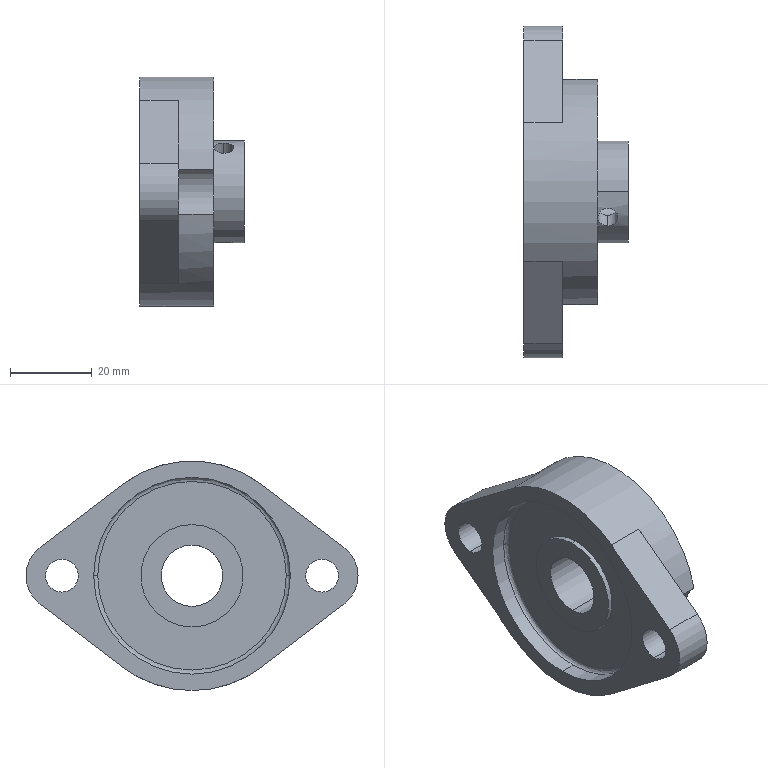Part | SolidWorks | features BaseBody 1 | 1 solid | 41 faces | box 25.5 x 81 x 56 mm | volume 35295 mm3 | cylinder 25 | plane 12 | spline 4 | commonest cylinder face diameters 4.917 x4 8 x4 25 x4 48 x4 56 x3 14 x2